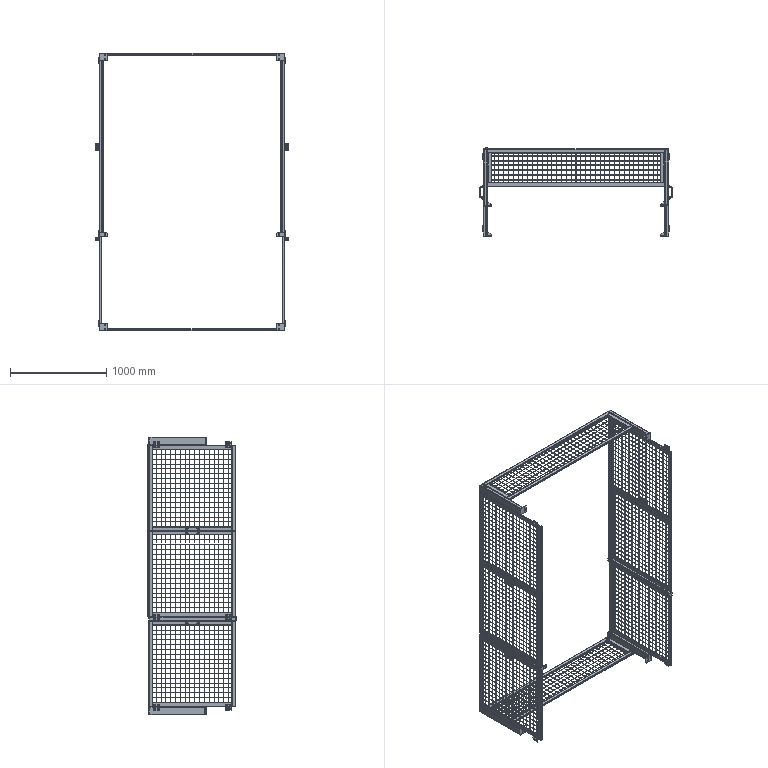Part | SolidWorks | 400 solids | 3314 faces | volume 13232952 mm3 | plane 1710 | cylinder 1484 | cone 116 | torus 4 | commonest cylinder face diameters 4 x576 6 x224 9 x136 6.8 x100 2 x96 8 x68